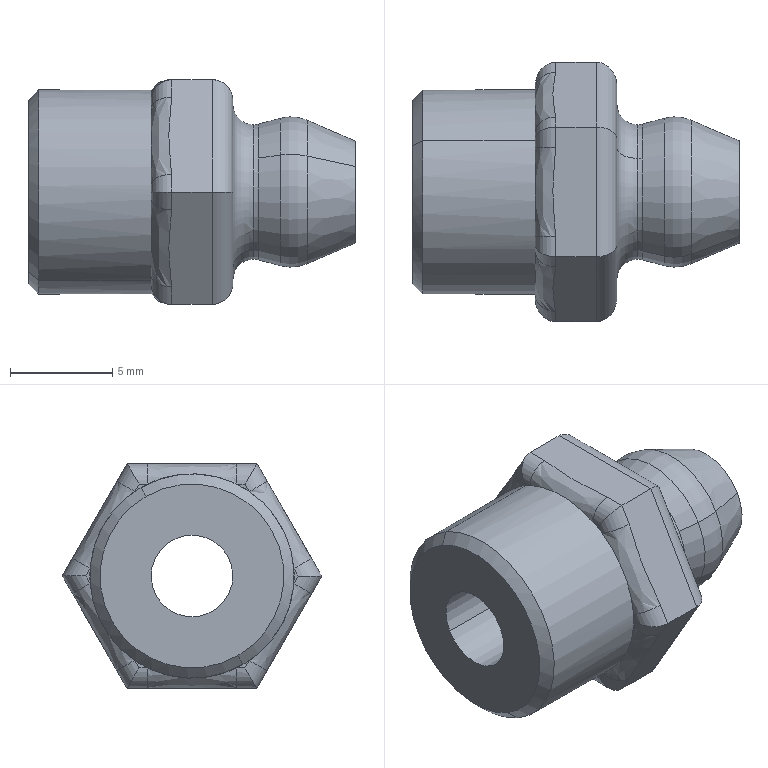Part | STEP file | Input 73 | 1 solid | 55 faces | box 16 x 12.702 x 11.006 mm | volume 882.434 mm3 | cylinder 22 | plane 15 | cone 6 | spline 6 | torus 4 | other 2 | commonest cylinder face diameters 2 x18 4 x2 10 x2